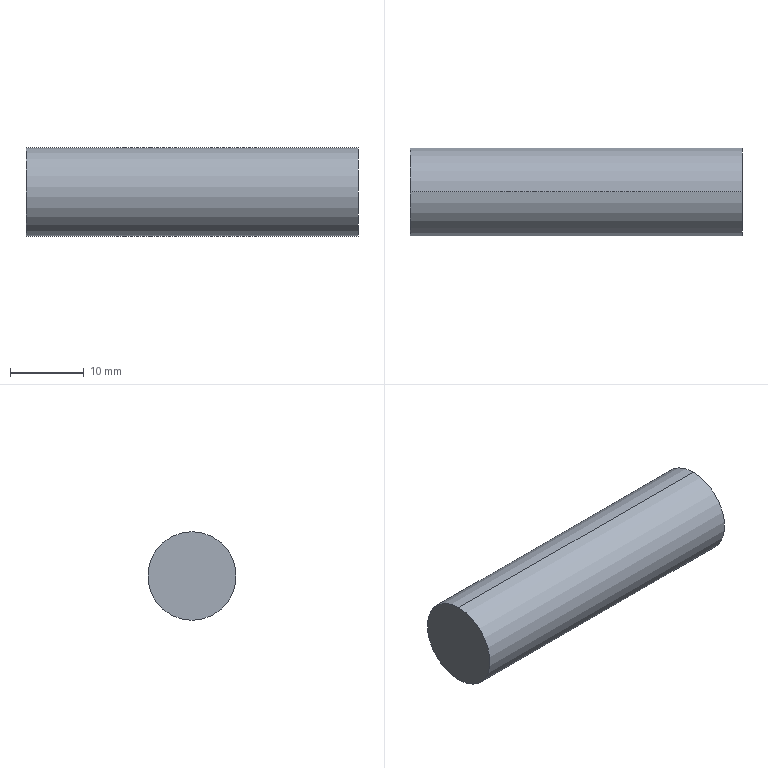Part | NX | features BREP 1 | 1 solid | 4 faces | box 45 x 12 x 12 mm | volume 5089 mm3 | cylinder 2 | plane 2 | commonest cylinder face diameters 12 x2
STEP:
#1=CARTESIAN_POINT('',(23.268,6.128,6.));
#2=VERTEX_POINT('',#1);
#3=CARTESIAN_POINT('',(23.268,6.128,-6.));
#4=VERTEX_POINT('',#3);
#5=CARTESIAN_POINT('',(23.268,6.128,0.));
#6=DIRECTION('',(-1.,0.,0.));
#7=DIRECTION('',(0.,0.,1.));
#8=AXIS2_PLACEMENT_3D('',#5,#6,#7);
#9=CIRCLE('',#8,6.);
#10=EDGE_CURVE('',#2,#4,#9,.T.);
#11=ORIENTED_EDGE('',*,*,#10,.T.);
#12=CARTESIAN_POINT('',(-21.732,6.128,-6.));
#13=VERTEX_POINT('',#12);
#14=CARTESIAN_POINT('',(-21.732,6.128,-6.));
#15=DIRECTION('',(-1.,0.,0.));
#16=VECTOR('',#15,1000.);
#17=LINE('',#14,#16);
#18=EDGE_CURVE('',#4,#13,#17,.T.);
#19=ORIENTED_EDGE('',*,*,#18,.T.);
#20=CARTESIAN_POINT('',(-21.732,6.128,6.));
#21=VERTEX_POINT('',#20);
#22=CARTESIAN_POINT('',(-21.732,6.128,0.));
#23=DIRECTION('',(-1.,0.,0.));
#24=DIRECTION('',(0.,0.,1.));
#25=AXIS2_PLACEMENT_3D('',#22,#23,#24);
#26=CIRCLE('',#25,6.);
#27=EDGE_CURVE('',#21,#13,#26,.T.);
#28=ORIENTED_EDGE('',*,*,#27,.F.);
#29=CARTESIAN_POINT('',(-21.732,6.128,6.));
#30=DIRECTION('',(-1.,0.,0.));
#31=VECTOR('',#30,1000.);
#32=LINE('',#29,#31);
#33=EDGE_CURVE('',#2,#21,#32,.T.);
#34=ORIENTED_EDGE('',*,*,#33,.F.);
#35=EDGE_LOOP('',(#11,#19,#28,#34));
#36=FACE_BOUND('',#35,.T.);
#37=CARTESIAN_POINT('',(-21.732,6.128,0.));
#38=DIRECTION('',(-1.,0.,0.));
#39=DIRECTION('',(0.,0.,-1.));
#40=AXIS2_PLACEMENT_3D('',#37,#38,#39);
#41=CYLINDRICAL_SURFACE('',#40,6.);
#42=ADVANCED_FACE('',(#36),#41,.T.);
#43=ORIENTED_EDGE('',*,*,#10,.F.);
#44=CARTESIAN_POINT('',(23.268,6.128,0.));
#45=DIRECTION('',(-1.,0.,0.));
#46=DIRECTION('',(0.,0.,1.));
#47=AXIS2_PLACEMENT_3D('',#44,#45,#46);
#48=CIRCLE('',#47,6.);
#49=EDGE_CURVE('',#4,#2,#48,.T.);
#50=ORIENTED_EDGE('',*,*,#49,.F.);
#51=EDGE_LOOP('',(#43,#50));
#52=FACE_BOUND('',#51,.T.);
#53=CARTESIAN_POINT('',(23.268,6.128,0.));
#54=DIRECTION('',(-1.,0.,0.));
#55=DIRECTION('',(0.,0.,-1.));
#56=AXIS2_PLACEMENT_3D('',#53,#54,#55);
#57=PLANE('',#56);
#58=ADVANCED_FACE('',(#52),#57,.F.);
#59=ORIENTED_EDGE('',*,*,#27,.T.);
#60=CARTESIAN_POINT('',(-21.732,6.128,0.));
#61=DIRECTION('',(-1.,0.,0.));
#62=DIRECTION('',(0.,0.,1.));
#63=AXIS2_PLACEMENT_3D('',#60,#61,#62);
#64=CIRCLE('',#63,6.);
#65=EDGE_CURVE('',#13,#21,#64,.T.);
#66=ORIENTED_EDGE('',*,*,#65,.T.);
#67=EDGE_LOOP('',(#59,#66));
#68=FACE_BOUND('',#67,.T.);
#69=CARTESIAN_POINT('',(-21.732,6.128,0.));
#70=DIRECTION('',(1.,0.,0.));
#71=DIRECTION('',(0.,-1.,0.));
#72=AXIS2_PLACEMENT_3D('',#69,#70,#71);
#73=PLANE('',#72);
#74=ADVANCED_FACE('',(#68),#73,.F.);
#75=ORIENTED_EDGE('',*,*,#18,.F.);
#76=ORIENTED_EDGE('',*,*,#49,.T.);
#77=ORIENTED_EDGE('',*,*,#33,.T.);
#78=ORIENTED_EDGE('',*,*,#65,.F.);
#79=EDGE_LOOP('',(#75,#76,#77,#78));
#80=FACE_BOUND('',#79,.T.);
#81=CARTESIAN_POINT('',(-21.732,6.128,0.));
#82=DIRECTION('',(-1.,0.,0.));
#83=DIRECTION('',(0.,0.,-1.));
#84=AXIS2_PLACEMENT_3D('',#81,#82,#83);
#85=CYLINDRICAL_SURFACE('',#84,6.);
#86=ADVANCED_FACE('',(#80),#85,.T.);
#87=CLOSED_SHELL('',(#42,#58,#74,#86));
#88=MANIFOLD_SOLID_BREP('',#87);
#89=(LENGTH_UNIT()NAMED_UNIT(*)SI_UNIT(.MILLI.,.METRE.));
#90=UNCERTAINTY_MEASURE_WITH_UNIT(LENGTH_MEASURE(0.00001),#89,'','');
#91=(NAMED_UNIT(*)PLANE_ANGLE_UNIT()SI_UNIT($,.RADIAN.));
#92=(NAMED_UNIT(*)SI_UNIT($,.STERADIAN.)SOLID_ANGLE_UNIT());
#93=(GEOMETRIC_REPRESENTATION_CONTEXT(3)GLOBAL_UNCERTAINTY_ASSIGNED_CONTEXT((#90))GLOBAL_UNIT_ASSIGNED_CONTEXT((#89,#91,#92))REPRESENTATION_CONTEXT('',''));
#94=ADVANCED_BREP_SHAPE_REPRESENTATION('',(#88),#93);